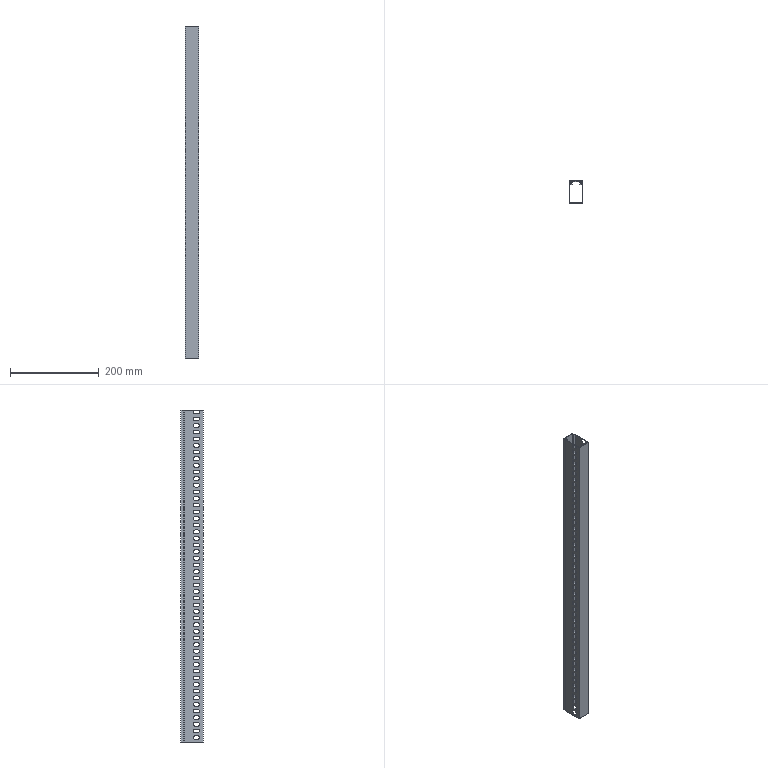Part | SolidWorks | features BaseBody 1 | 1 solid | 426 faces | box 30 x 50 x 750 mm | volume 122173 mm3 | plane 226 | cylinder 200 | commonest cylinder face diameters 8 x200